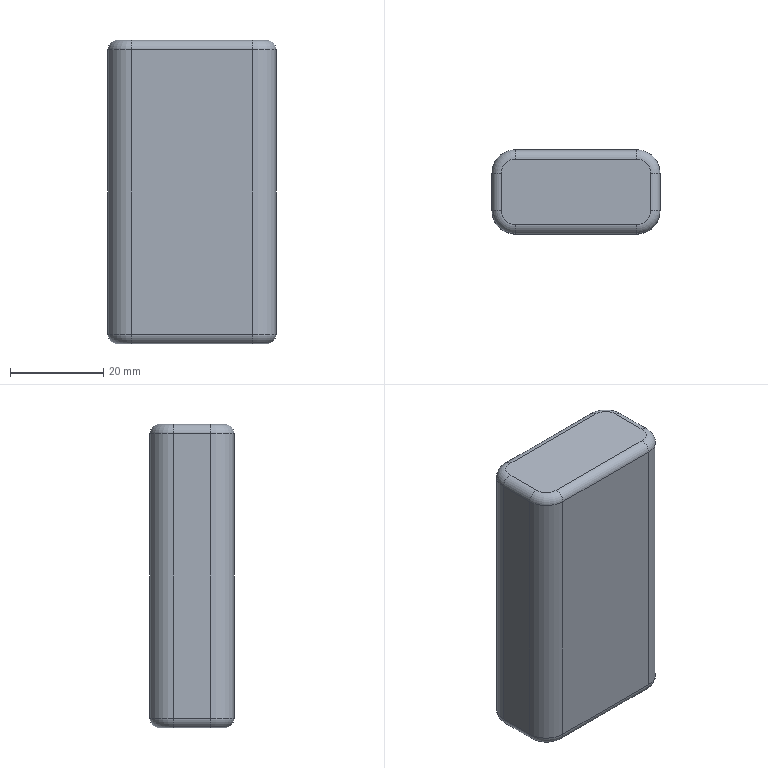Part | SolidWorks | features Fillet 2, Extrusion 1 | 1 solid | 26 faces | box 36 x 18 x 65 mm | volume 40559 mm3 | cylinder 12 | torus 8 | plane 6 | commonest cylinder face diameters 4 x8 10 x4
STEP:
#1=CARTESIAN_POINT('',(18.,-4.,63.));
#2=VERTEX_POINT('',#1);
#3=CARTESIAN_POINT('',(18.,-4.,2.));
#4=VERTEX_POINT('',#3);
#5=CARTESIAN_POINT('',(18.,-4.,65.));
#6=DIRECTION('',(0.,0.,-1.));
#7=VECTOR('',#6,1000.);
#8=LINE('',#5,#7);
#9=EDGE_CURVE('',#2,#4,#8,.T.);
#10=ORIENTED_EDGE('',*,*,#9,.T.);
#11=CARTESIAN_POINT('',(18.,4.,2.));
#12=VERTEX_POINT('',#11);
#13=CARTESIAN_POINT('',(18.,9.,2.));
#14=DIRECTION('',(0.,1.,0.));
#15=VECTOR('',#14,1000.);
#16=LINE('',#13,#15);
#17=EDGE_CURVE('',#4,#12,#16,.T.);
#18=ORIENTED_EDGE('',*,*,#17,.T.);
#19=CARTESIAN_POINT('',(18.,4.,63.));
#20=VERTEX_POINT('',#19);
#21=CARTESIAN_POINT('',(18.,4.,65.));
#22=DIRECTION('',(0.,0.,1.));
#23=VECTOR('',#22,1000.);
#24=LINE('',#21,#23);
#25=EDGE_CURVE('',#12,#20,#24,.T.);
#26=ORIENTED_EDGE('',*,*,#25,.T.);
#27=CARTESIAN_POINT('',(18.,-4.,63.));
#28=DIRECTION('',(0.,-1.,0.));
#29=VECTOR('',#28,1000.);
#30=LINE('',#27,#29);
#31=EDGE_CURVE('',#20,#2,#30,.T.);
#32=ORIENTED_EDGE('',*,*,#31,.T.);
#33=EDGE_LOOP('',(#10,#18,#26,#32));
#34=FACE_OUTER_BOUND('',#33,.T.);
#35=CARTESIAN_POINT('',(18.,9.,65.));
#36=DIRECTION('',(-1.,0.,0.));
#37=DIRECTION('',(0.,0.,1.));
#38=AXIS2_PLACEMENT_3D('',#35,#36,#37);
#39=PLANE('',#38);
#40=ADVANCED_FACE('',(#34),#39,.F.);
#41=CARTESIAN_POINT('',(13.,9.,63.));
#42=VERTEX_POINT('',#41);
#43=CARTESIAN_POINT('',(13.,9.,2.));
#44=VERTEX_POINT('',#43);
#45=CARTESIAN_POINT('',(13.,9.,65.));
#46=DIRECTION('',(0.,0.,-1.));
#47=VECTOR('',#46,1000.);
#48=LINE('',#45,#47);
#49=EDGE_CURVE('',#42,#44,#48,.T.);
#50=ORIENTED_EDGE('',*,*,#49,.T.);
#51=CARTESIAN_POINT('',(-13.,9.,2.));
#52=VERTEX_POINT('',#51);
#53=CARTESIAN_POINT('',(-18.,9.,2.));
#54=DIRECTION('',(-1.,0.,0.));
#55=VECTOR('',#54,1000.);
#56=LINE('',#53,#55);
#57=EDGE_CURVE('',#44,#52,#56,.T.);
#58=ORIENTED_EDGE('',*,*,#57,.T.);
#59=CARTESIAN_POINT('',(-13.,9.,63.));
#60=VERTEX_POINT('',#59);
#61=CARTESIAN_POINT('',(-13.,9.,65.));
#62=DIRECTION('',(0.,0.,1.));
#63=VECTOR('',#62,1000.);
#64=LINE('',#61,#63);
#65=EDGE_CURVE('',#52,#60,#64,.T.);
#66=ORIENTED_EDGE('',*,*,#65,.T.);
#67=CARTESIAN_POINT('',(13.,9.,63.));
#68=DIRECTION('',(1.,0.,0.));
#69=VECTOR('',#68,1000.);
#70=LINE('',#67,#69);
#71=EDGE_CURVE('',#60,#42,#70,.T.);
#72=ORIENTED_EDGE('',*,*,#71,.T.);
#73=EDGE_LOOP('',(#50,#58,#66,#72));
#74=FACE_OUTER_BOUND('',#73,.T.);
#75=CARTESIAN_POINT('',(-18.,9.,65.));
#76=DIRECTION('',(0.,-1.,0.));
#77=DIRECTION('',(0.,0.,-1.));
#78=AXIS2_PLACEMENT_3D('',#75,#76,#77);
#79=PLANE('',#78);
#80=ADVANCED_FACE('',(#74),#79,.F.);
#81=CARTESIAN_POINT('',(-18.,4.,63.));
#82=VERTEX_POINT('',#81);
#83=CARTESIAN_POINT('',(-18.,4.,2.));
#84=VERTEX_POINT('',#83);
#85=CARTESIAN_POINT('',(-18.,4.,65.));
#86=DIRECTION('',(0.,0.,-1.));
#87=VECTOR('',#86,1000.);
#88=LINE('',#85,#87);
#89=EDGE_CURVE('',#82,#84,#88,.T.);
#90=ORIENTED_EDGE('',*,*,#89,.T.);
#91=CARTESIAN_POINT('',(-18.,-4.,2.));
#92=VERTEX_POINT('',#91);
#93=CARTESIAN_POINT('',(-18.,9.,2.));
#94=DIRECTION('',(0.,-1.,0.));
#95=VECTOR('',#94,1000.);
#96=LINE('',#93,#95);
#97=EDGE_CURVE('',#84,#92,#96,.T.);
#98=ORIENTED_EDGE('',*,*,#97,.T.);
#99=CARTESIAN_POINT('',(-18.,-4.,63.));
#100=VERTEX_POINT('',#99);
#101=CARTESIAN_POINT('',(-18.,-4.,65.));
#102=DIRECTION('',(0.,0.,1.));
#103=VECTOR('',#102,1000.);
#104=LINE('',#101,#103);
#105=EDGE_CURVE('',#92,#100,#104,.T.);
#106=ORIENTED_EDGE('',*,*,#105,.T.);
#107=CARTESIAN_POINT('',(-18.,4.,63.));
#108=DIRECTION('',(0.,1.,0.));
#109=VECTOR('',#108,1000.);
#110=LINE('',#107,#109);
#111=EDGE_CURVE('',#100,#82,#110,.T.);
#112=ORIENTED_EDGE('',*,*,#111,.T.);
#113=EDGE_LOOP('',(#90,#98,#106,#112));
#114=FACE_OUTER_BOUND('',#113,.T.);
#115=CARTESIAN_POINT('',(-18.,9.,65.));
#116=DIRECTION('',(1.,0.,0.));
#117=DIRECTION('',(0.,0.,-1.));
#118=AXIS2_PLACEMENT_3D('',#115,#116,#117);
#119=PLANE('',#118);
#120=ADVANCED_FACE('',(#114),#119,.F.);
#121=CARTESIAN_POINT('',(-13.,-9.,63.));
#122=VERTEX_POINT('',#121);
#123=CARTESIAN_POINT('',(-13.,-9.,2.));
#124=VERTEX_POINT('',#123);
#125=CARTESIAN_POINT('',(-13.,-9.,65.));
#126=DIRECTION('',(0.,0.,-1.));
#127=VECTOR('',#126,1000.);
#128=LINE('',#125,#127);
#129=EDGE_CURVE('',#122,#124,#128,.T.);
#130=ORIENTED_EDGE('',*,*,#129,.T.);
#131=CARTESIAN_POINT('',(13.,-9.,2.));
#132=VERTEX_POINT('',#131);
#133=CARTESIAN_POINT('',(-18.,-9.,2.));
#134=DIRECTION('',(1.,0.,0.));
#135=VECTOR('',#134,1000.);
#136=LINE('',#133,#135);
#137=EDGE_CURVE('',#124,#132,#136,.T.);
#138=ORIENTED_EDGE('',*,*,#137,.T.);
#139=CARTESIAN_POINT('',(13.,-9.,63.));
#140=VERTEX_POINT('',#139);
#141=CARTESIAN_POINT('',(13.,-9.,65.));
#142=DIRECTION('',(0.,0.,1.));
#143=VECTOR('',#142,1000.);
#144=LINE('',#141,#143);
#145=EDGE_CURVE('',#132,#140,#144,.T.);
#146=ORIENTED_EDGE('',*,*,#145,.T.);
#147=CARTESIAN_POINT('',(-13.,-9.,63.));
#148=DIRECTION('',(-1.,0.,0.));
#149=VECTOR('',#148,1000.);
#150=LINE('',#147,#149);
#151=EDGE_CURVE('',#140,#122,#150,.T.);
#152=ORIENTED_EDGE('',*,*,#151,.T.);
#153=EDGE_LOOP('',(#130,#138,#146,#152));
#154=FACE_OUTER_BOUND('',#153,.T.);
#155=CARTESIAN_POINT('',(-18.,-9.,65.));
#156=DIRECTION('',(0.,1.,0.));
#157=DIRECTION('',(0.,0.,1.));
#158=AXIS2_PLACEMENT_3D('',#155,#156,#157);
#159=PLANE('',#158);
#160=ADVANCED_FACE('',(#154),#159,.F.);
#161=CARTESIAN_POINT('',(13.,7.,65.));
#162=VERTEX_POINT('',#161);
#163=CARTESIAN_POINT('',(-13.,7.,65.));
#164=VERTEX_POINT('',#163);
#165=CARTESIAN_POINT('',(-13.,7.,65.));
#166=DIRECTION('',(-1.,0.,0.));
#167=VECTOR('',#166,1000.);
#168=LINE('',#165,#167);
#169=EDGE_CURVE('',#162,#164,#168,.T.);
#170=ORIENTED_EDGE('',*,*,#169,.T.);
#171=CARTESIAN_POINT('',(-16.,4.,65.));
#172=VERTEX_POINT('',#171);
#173=CARTESIAN_POINT('',(-13.,4.,65.));
#174=DIRECTION('',(0.,0.,1.));
#175=DIRECTION('',(1.,0.,0.));
#176=AXIS2_PLACEMENT_3D('',#173,#174,#175);
#177=CIRCLE('',#176,3.);
#178=EDGE_CURVE('',#164,#172,#177,.T.);
#179=ORIENTED_EDGE('',*,*,#178,.T.);
#180=CARTESIAN_POINT('',(-16.,-4.,65.));
#181=VERTEX_POINT('',#180);
#182=CARTESIAN_POINT('',(-16.,-4.,65.));
#183=DIRECTION('',(0.,-1.,0.));
#184=VECTOR('',#183,1000.);
#185=LINE('',#182,#184);
#186=EDGE_CURVE('',#172,#181,#185,.T.);
#187=ORIENTED_EDGE('',*,*,#186,.T.);
#188=CARTESIAN_POINT('',(-13.,-7.,65.));
#189=VERTEX_POINT('',#188);
#190=CARTESIAN_POINT('',(-13.,-4.,65.));
#191=DIRECTION('',(0.,0.,1.));
#192=DIRECTION('',(1.,0.,0.));
#193=AXIS2_PLACEMENT_3D('',#190,#191,#192);
#194=CIRCLE('',#193,3.);
#195=EDGE_CURVE('',#181,#189,#194,.T.);
#196=ORIENTED_EDGE('',*,*,#195,.T.);
#197=CARTESIAN_POINT('',(13.,-7.,65.));
#198=VERTEX_POINT('',#197);
#199=CARTESIAN_POINT('',(13.,-7.,65.));
#200=DIRECTION('',(1.,0.,0.));
#201=VECTOR('',#200,1000.);
#202=LINE('',#199,#201);
#203=EDGE_CURVE('',#189,#198,#202,.T.);
#204=ORIENTED_EDGE('',*,*,#203,.T.);
#205=CARTESIAN_POINT('',(16.,-4.,65.));
#206=VERTEX_POINT('',#205);
#207=CARTESIAN_POINT('',(13.,-4.,65.));
#208=DIRECTION('',(0.,0.,1.));
#209=DIRECTION('',(1.,0.,0.));
#210=AXIS2_PLACEMENT_3D('',#207,#208,#209);
#211=CIRCLE('',#210,3.);
#212=EDGE_CURVE('',#198,#206,#211,.T.);
#213=ORIENTED_EDGE('',*,*,#212,.T.);
#214=CARTESIAN_POINT('',(16.,4.,65.));
#215=VERTEX_POINT('',#214);
#216=CARTESIAN_POINT('',(16.,4.,65.));
#217=DIRECTION('',(0.,1.,0.));
#218=VECTOR('',#217,1000.);
#219=LINE('',#216,#218);
#220=EDGE_CURVE('',#206,#215,#219,.T.);
#221=ORIENTED_EDGE('',*,*,#220,.T.);
#222=CARTESIAN_POINT('',(13.,4.,65.));
#223=DIRECTION('',(0.,0.,1.));
#224=DIRECTION('',(1.,0.,0.));
#225=AXIS2_PLACEMENT_3D('',#222,#223,#224);
#226=CIRCLE('',#225,3.);
#227=EDGE_CURVE('',#215,#162,#226,.T.);
#228=ORIENTED_EDGE('',*,*,#227,.T.);
#229=EDGE_LOOP('',(#170,#179,#187,#196,#204,#213,#221,#228));
#230=FACE_OUTER_BOUND('',#229,.T.);
#231=CARTESIAN_POINT('',(0.,0.,65.));
#232=DIRECTION('',(0.,0.,1.));
#233=DIRECTION('',(1.,0.,0.));
#234=AXIS2_PLACEMENT_3D('',#231,#232,#233);
#235=PLANE('',#234);
#236=ADVANCED_FACE('',(#230),#235,.T.);
#237=CARTESIAN_POINT('',(16.,4.,0.));
#238=VERTEX_POINT('',#237);
#239=CARTESIAN_POINT('',(16.,-4.,0.));
#240=VERTEX_POINT('',#239);
#241=CARTESIAN_POINT('',(16.,0.,0.));
#242=DIRECTION('',(0.,-1.,0.));
#243=VECTOR('',#242,1000.);
#244=LINE('',#241,#243);
#245=EDGE_CURVE('',#238,#240,#244,.T.);
#246=ORIENTED_EDGE('',*,*,#245,.T.);
#247=CARTESIAN_POINT('',(13.,-7.,0.));
#248=VERTEX_POINT('',#247);
#249=CARTESIAN_POINT('',(13.,-4.,0.));
#250=DIRECTION('',(0.,0.,-1.));
#251=DIRECTION('',(1.,0.,0.));
#252=AXIS2_PLACEMENT_3D('',#249,#250,#251);
#253=CIRCLE('',#252,3.);
#254=EDGE_CURVE('',#240,#248,#253,.T.);
#255=ORIENTED_EDGE('',*,*,#254,.T.);
#256=CARTESIAN_POINT('',(-13.,-7.,0.));
#257=VERTEX_POINT('',#256);
#258=CARTESIAN_POINT('',(0.,-7.,0.));
#259=DIRECTION('',(-1.,0.,0.));
#260=VECTOR('',#259,1000.);
#261=LINE('',#258,#260);
#262=EDGE_CURVE('',#248,#257,#261,.T.);
#263=ORIENTED_EDGE('',*,*,#262,.T.);
#264=CARTESIAN_POINT('',(-16.,-4.,0.));
#265=VERTEX_POINT('',#264);
#266=CARTESIAN_POINT('',(-13.,-4.,0.));
#267=DIRECTION('',(0.,0.,-1.));
#268=DIRECTION('',(1.,0.,0.));
#269=AXIS2_PLACEMENT_3D('',#266,#267,#268);
#270=CIRCLE('',#269,3.);
#271=EDGE_CURVE('',#257,#265,#270,.T.);
#272=ORIENTED_EDGE('',*,*,#271,.T.);
#273=CARTESIAN_POINT('',(-16.,4.,0.));
#274=VERTEX_POINT('',#273);
#275=CARTESIAN_POINT('',(-16.,0.,0.));
#276=DIRECTION('',(0.,1.,0.));
#277=VECTOR('',#276,1000.);
#278=LINE('',#275,#277);
#279=EDGE_CURVE('',#265,#274,#278,.T.);
#280=ORIENTED_EDGE('',*,*,#279,.T.);
#281=CARTESIAN_POINT('',(-13.,7.,0.));
#282=VERTEX_POINT('',#281);
#283=CARTESIAN_POINT('',(-13.,4.,0.));
#284=DIRECTION('',(0.,0.,-1.));
#285=DIRECTION('',(1.,0.,0.));
#286=AXIS2_PLACEMENT_3D('',#283,#284,#285);
#287=CIRCLE('',#286,3.);
#288=EDGE_CURVE('',#274,#282,#287,.T.);
#289=ORIENTED_EDGE('',*,*,#288,.T.);
#290=CARTESIAN_POINT('',(13.,7.,0.));
#291=VERTEX_POINT('',#290);
#292=CARTESIAN_POINT('',(0.,7.,0.));
#293=DIRECTION('',(1.,0.,0.));
#294=VECTOR('',#293,1000.);
#295=LINE('',#292,#294);
#296=EDGE_CURVE('',#282,#291,#295,.T.);
#297=ORIENTED_EDGE('',*,*,#296,.T.);
#298=CARTESIAN_POINT('',(13.,4.,0.));
#299=DIRECTION('',(0.,0.,-1.));
#300=DIRECTION('',(1.,0.,0.));
#301=AXIS2_PLACEMENT_3D('',#298,#299,#300);
#302=CIRCLE('',#301,3.);
#303=EDGE_CURVE('',#291,#238,#302,.T.);
#304=ORIENTED_EDGE('',*,*,#303,.T.);
#305=EDGE_LOOP('',(#246,#255,#263,#272,#280,#289,#297,#304));
#306=FACE_OUTER_BOUND('',#305,.T.);
#307=CARTESIAN_POINT('',(0.,0.,0.));
#308=DIRECTION('',(0.,0.,1.));
#309=DIRECTION('',(1.,0.,0.));
#310=AXIS2_PLACEMENT_3D('',#307,#308,#309);
#311=PLANE('',#310);
#312=ADVANCED_FACE('',(#306),#311,.F.);
#313=ORIENTED_EDGE('',*,*,#105,.F.);
#314=CARTESIAN_POINT('',(-13.,-4.,2.));
#315=DIRECTION('',(0.,0.,1.));
#316=DIRECTION('',(1.,0.,0.));
#317=AXIS2_PLACEMENT_3D('',#314,#315,#316);
#318=CIRCLE('',#317,5.);
#319=EDGE_CURVE('',#92,#124,#318,.T.);
#320=ORIENTED_EDGE('',*,*,#319,.T.);
#321=ORIENTED_EDGE('',*,*,#129,.F.);
#322=CARTESIAN_POINT('',(-13.,-4.,63.));
#323=DIRECTION('',(0.,0.,-1.));
#324=DIRECTION('',(1.,0.,0.));
#325=AXIS2_PLACEMENT_3D('',#322,#323,#324);
#326=CIRCLE('',#325,5.);
#327=EDGE_CURVE('',#122,#100,#326,.T.);
#328=ORIENTED_EDGE('',*,*,#327,.T.);
#329=EDGE_LOOP('',(#313,#320,#321,#328));
#330=FACE_OUTER_BOUND('',#329,.T.);
#331=CARTESIAN_POINT('',(-13.,-4.,65.));
#332=DIRECTION('',(0.,0.,-1.));
#333=DIRECTION('',(-1.,0.,0.));
#334=AXIS2_PLACEMENT_3D('',#331,#332,#333);
#335=CYLINDRICAL_SURFACE('',#334,5.);
#336=ADVANCED_FACE('',(#330),#335,.T.);
#337=ORIENTED_EDGE('',*,*,#65,.F.);
#338=CARTESIAN_POINT('',(-13.,4.,2.));
#339=DIRECTION('',(0.,0.,1.));
#340=DIRECTION('',(1.,0.,0.));
#341=AXIS2_PLACEMENT_3D('',#338,#339,#340);
#342=CIRCLE('',#341,5.);
#343=EDGE_CURVE('',#52,#84,#342,.T.);
#344=ORIENTED_EDGE('',*,*,#343,.T.);
#345=ORIENTED_EDGE('',*,*,#89,.F.);
#346=CARTESIAN_POINT('',(-13.,4.,63.));
#347=DIRECTION('',(0.,0.,-1.));
#348=DIRECTION('',(1.,0.,0.));
#349=AXIS2_PLACEMENT_3D('',#346,#347,#348);
#350=CIRCLE('',#349,5.);
#351=EDGE_CURVE('',#82,#60,#350,.T.);
#352=ORIENTED_EDGE('',*,*,#351,.T.);
#353=EDGE_LOOP('',(#337,#344,#345,#352));
#354=FACE_OUTER_BOUND('',#353,.T.);
#355=CARTESIAN_POINT('',(-13.,4.,65.));
#356=DIRECTION('',(0.,0.,-1.));
#357=DIRECTION('',(-1.,0.,0.));
#358=AXIS2_PLACEMENT_3D('',#355,#356,#357);
#359=CYLINDRICAL_SURFACE('',#358,5.);
#360=ADVANCED_FACE('',(#354),#359,.T.);
#361=ORIENTED_EDGE('',*,*,#145,.F.);
#362=CARTESIAN_POINT('',(13.,-4.,2.));
#363=DIRECTION('',(0.,0.,1.));
#364=DIRECTION('',(1.,0.,0.));
#365=AXIS2_PLACEMENT_3D('',#362,#363,#364);
#366=CIRCLE('',#365,5.);
#367=EDGE_CURVE('',#132,#4,#366,.T.);
#368=ORIENTED_EDGE('',*,*,#367,.T.);
#369=ORIENTED_EDGE('',*,*,#9,.F.);
#370=CARTESIAN_POINT('',(13.,-4.,63.));
#371=DIRECTION('',(0.,0.,-1.));
#372=DIRECTION('',(1.,0.,0.));
#373=AXIS2_PLACEMENT_3D('',#370,#371,#372);
#374=CIRCLE('',#373,5.);
#375=EDGE_CURVE('',#2,#140,#374,.T.);
#376=ORIENTED_EDGE('',*,*,#375,.T.);
#377=EDGE_LOOP('',(#361,#368,#369,#376));
#378=FACE_OUTER_BOUND('',#377,.T.);
#379=CARTESIAN_POINT('',(13.,-4.,65.));
#380=DIRECTION('',(0.,0.,-1.));
#381=DIRECTION('',(-1.,0.,0.));
#382=AXIS2_PLACEMENT_3D('',#379,#380,#381);
#383=CYLINDRICAL_SURFACE('',#382,5.);
#384=ADVANCED_FACE('',(#378),#383,.T.);
#385=ORIENTED_EDGE('',*,*,#25,.F.);
#386=CARTESIAN_POINT('',(13.,4.,2.));
#387=DIRECTION('',(0.,0.,1.));
#388=DIRECTION('',(1.,0.,0.));
#389=AXIS2_PLACEMENT_3D('',#386,#387,#388);
#390=CIRCLE('',#389,5.);
#391=EDGE_CURVE('',#12,#44,#390,.T.);
#392=ORIENTED_EDGE('',*,*,#391,.T.);
#393=ORIENTED_EDGE('',*,*,#49,.F.);
#394=CARTESIAN_POINT('',(13.,4.,63.));
#395=DIRECTION('',(0.,0.,-1.));
#396=DIRECTION('',(1.,0.,0.));
#397=AXIS2_PLACEMENT_3D('',#394,#395,#396);
#398=CIRCLE('',#397,5.);
#399=EDGE_CURVE('',#42,#20,#398,.T.);
#400=ORIENTED_EDGE('',*,*,#399,.T.);
#401=EDGE_LOOP('',(#385,#392,#393,#400));
#402=FACE_OUTER_BOUND('',#401,.T.);
#403=CARTESIAN_POINT('',(13.,4.,65.));
#404=DIRECTION('',(0.,0.,-1.));
#405=DIRECTION('',(-1.,0.,0.));
#406=AXIS2_PLACEMENT_3D('',#403,#404,#405);
#407=CYLINDRICAL_SURFACE('',#406,5.);
#408=ADVANCED_FACE('',(#402),#407,.T.);
#409=CARTESIAN_POINT('',(-16.,4.,2.));
#410=DIRECTION('',(0.,-1.,0.));
#411=DIRECTION('',(0.,0.,-1.));
#412=AXIS2_PLACEMENT_3D('',#409,#410,#411);
#413=CIRCLE('',#412,2.);
#414=EDGE_CURVE('',#84,#274,#413,.T.);
#415=ORIENTED_EDGE('',*,*,#414,.F.);
#416=ORIENTED_EDGE('',*,*,#343,.F.);
#417=CARTESIAN_POINT('',(-13.,7.,2.));
#418=DIRECTION('',(1.,0.,0.));
#419=DIRECTION('',(0.,0.,-1.));
#420=AXIS2_PLACEMENT_3D('',#417,#418,#419);
#421=CIRCLE('',#420,2.);
#422=EDGE_CURVE('',#282,#52,#421,.T.);
#423=ORIENTED_EDGE('',*,*,#422,.F.);
#424=ORIENTED_EDGE('',*,*,#288,.F.);
#425=EDGE_LOOP('',(#415,#416,#423,#424));
#426=FACE_OUTER_BOUND('',#425,.T.);
#427=CARTESIAN_POINT('',(-13.,4.,2.));
#428=DIRECTION('',(0.,0.,1.));
#429=DIRECTION('',(1.,0.,0.));
#430=AXIS2_PLACEMENT_3D('',#427,#428,#429);
#431=TOROIDAL_SURFACE('',#430,3.,2.);
#432=ADVANCED_FACE('',(#426),#431,.T.);
#433=ORIENTED_EDGE('',*,*,#422,.T.);
#434=ORIENTED_EDGE('',*,*,#57,.F.);
#435=CARTESIAN_POINT('',(13.,7.,2.));
#436=DIRECTION('',(1.,0.,0.));
#437=DIRECTION('',(0.,0.,-1.));
#438=AXIS2_PLACEMENT_3D('',#435,#436,#437);
#439=CIRCLE('',#438,2.);
#440=EDGE_CURVE('',#291,#44,#439,.T.);
#441=ORIENTED_EDGE('',*,*,#440,.F.);
#442=ORIENTED_EDGE('',*,*,#296,.F.);
#443=EDGE_LOOP('',(#433,#434,#441,#442));
#444=FACE_OUTER_BOUND('',#443,.T.);
#445=CARTESIAN_POINT('',(-18.,7.,2.));
#446=DIRECTION('',(-1.,0.,0.));
#447=DIRECTION('',(0.,0.,1.));
#448=AXIS2_PLACEMENT_3D('',#445,#446,#447);
#449=CYLINDRICAL_SURFACE('',#448,2.);
#450=ADVANCED_FACE('',(#444),#449,.T.);
#451=ORIENTED_EDGE('',*,*,#414,.T.);
#452=ORIENTED_EDGE('',*,*,#279,.F.);
#453=CARTESIAN_POINT('',(-16.,-4.,2.));
#454=DIRECTION('',(0.,-1.,0.));
#455=DIRECTION('',(0.,0.,-1.));
#456=AXIS2_PLACEMENT_3D('',#453,#454,#455);
#457=CIRCLE('',#456,2.);
#458=EDGE_CURVE('',#92,#265,#457,.T.);
#459=ORIENTED_EDGE('',*,*,#458,.F.);
#460=ORIENTED_EDGE('',*,*,#97,.F.);
#461=EDGE_LOOP('',(#451,#452,#459,#460));
#462=FACE_OUTER_BOUND('',#461,.T.);
#463=CARTESIAN_POINT('',(-16.,9.,2.));
#464=DIRECTION('',(0.,-1.,0.));
#465=DIRECTION('',(0.,0.,-1.));
#466=AXIS2_PLACEMENT_3D('',#463,#464,#465);
#467=CYLINDRICAL_SURFACE('',#466,2.);
#468=ADVANCED_FACE('',(#462),#467,.T.);
#469=ORIENTED_EDGE('',*,*,#440,.T.);
#470=ORIENTED_EDGE('',*,*,#391,.F.);
#471=CARTESIAN_POINT('',(16.,4.,2.));
#472=DIRECTION('',(0.,-1.,0.));
#473=DIRECTION('',(0.,0.,-1.));
#474=AXIS2_PLACEMENT_3D('',#471,#472,#473);
#475=CIRCLE('',#474,2.);
#476=EDGE_CURVE('',#238,#12,#475,.T.);
#477=ORIENTED_EDGE('',*,*,#476,.F.);
#478=ORIENTED_EDGE('',*,*,#303,.F.);
#479=EDGE_LOOP('',(#469,#470,#477,#478));
#480=FACE_OUTER_BOUND('',#479,.T.);
#481=CARTESIAN_POINT('',(13.,4.,2.));
#482=DIRECTION('',(0.,0.,1.));
#483=DIRECTION('',(1.,0.,0.));
#484=AXIS2_PLACEMENT_3D('',#481,#482,#483);
#485=TOROIDAL_SURFACE('',#484,3.,2.);
#486=ADVANCED_FACE('',(#480),#485,.T.);
#487=ORIENTED_EDGE('',*,*,#458,.T.);
#488=ORIENTED_EDGE('',*,*,#271,.F.);
#489=CARTESIAN_POINT('',(-13.,-7.,2.));
#490=DIRECTION('',(1.,0.,0.));
#491=DIRECTION('',(0.,0.,-1.));
#492=AXIS2_PLACEMENT_3D('',#489,#490,#491);
#493=CIRCLE('',#492,2.);
#494=EDGE_CURVE('',#124,#257,#493,.T.);
#495=ORIENTED_EDGE('',*,*,#494,.F.);
#496=ORIENTED_EDGE('',*,*,#319,.F.);
#497=EDGE_LOOP('',(#487,#488,#495,#496));
#498=FACE_OUTER_BOUND('',#497,.T.);
#499=CARTESIAN_POINT('',(-13.,-4.,2.));
#500=DIRECTION('',(0.,0.,1.));
#501=DIRECTION('',(1.,0.,0.));
#502=AXIS2_PLACEMENT_3D('',#499,#500,#501);
#503=TOROIDAL_SURFACE('',#502,3.,2.);
#504=ADVANCED_FACE('',(#498),#503,.T.);
#505=ORIENTED_EDGE('',*,*,#476,.T.);
#506=ORIENTED_EDGE('',*,*,#17,.F.);
#507=CARTESIAN_POINT('',(16.,-4.,2.));
#508=DIRECTION('',(0.,-1.,0.));
#509=DIRECTION('',(0.,0.,-1.));
#510=AXIS2_PLACEMENT_3D('',#507,#508,#509);
#511=CIRCLE('',#510,2.);
#512=EDGE_CURVE('',#240,#4,#511,.T.);
#513=ORIENTED_EDGE('',*,*,#512,.F.);
#514=ORIENTED_EDGE('',*,*,#245,.F.);
#515=EDGE_LOOP('',(#505,#506,#513,#514));
#516=FACE_OUTER_BOUND('',#515,.T.);
#517=CARTESIAN_POINT('',(16.,9.,2.));
#518=DIRECTION('',(0.,1.,0.));
#519=DIRECTION('',(0.,0.,1.));
#520=AXIS2_PLACEMENT_3D('',#517,#518,#519);
#521=CYLINDRICAL_SURFACE('',#520,2.);
#522=ADVANCED_FACE('',(#516),#521,.T.);
#523=ORIENTED_EDGE('',*,*,#494,.T.);
#524=ORIENTED_EDGE('',*,*,#262,.F.);
#525=CARTESIAN_POINT('',(13.,-7.,2.));
#526=DIRECTION('',(1.,0.,0.));
#527=DIRECTION('',(0.,0.,-1.));
#528=AXIS2_PLACEMENT_3D('',#525,#526,#527);
#529=CIRCLE('',#528,2.);
#530=EDGE_CURVE('',#132,#248,#529,.T.);
#531=ORIENTED_EDGE('',*,*,#530,.F.);
#532=ORIENTED_EDGE('',*,*,#137,.F.);
#533=EDGE_LOOP('',(#523,#524,#531,#532));
#534=FACE_OUTER_BOUND('',#533,.T.);
#535=CARTESIAN_POINT('',(-18.,-7.,2.));
#536=DIRECTION('',(1.,0.,0.));
#537=DIRECTION('',(0.,0.,-1.));
#538=AXIS2_PLACEMENT_3D('',#535,#536,#537);
#539=CYLINDRICAL_SURFACE('',#538,2.);
#540=ADVANCED_FACE('',(#534),#539,.T.);
#541=ORIENTED_EDGE('',*,*,#512,.T.);
#542=ORIENTED_EDGE('',*,*,#367,.F.);
#543=ORIENTED_EDGE('',*,*,#530,.T.);
#544=ORIENTED_EDGE('',*,*,#254,.F.);
#545=EDGE_LOOP('',(#541,#542,#543,#544));
#546=FACE_OUTER_BOUND('',#545,.T.);
#547=CARTESIAN_POINT('',(13.,-4.,2.));
#548=DIRECTION('',(0.,0.,1.));
#549=DIRECTION('',(1.,0.,0.));
#550=AXIS2_PLACEMENT_3D('',#547,#548,#549);
#551=TOROIDAL_SURFACE('',#550,3.,2.);
#552=ADVANCED_FACE('',(#546),#551,.T.);
#553=CARTESIAN_POINT('',(13.,-7.,63.));
#554=DIRECTION('',(-1.,0.,0.));
#555=DIRECTION('',(0.,0.,1.));
#556=AXIS2_PLACEMENT_3D('',#553,#554,#555);
#557=CIRCLE('',#556,2.);
#558=EDGE_CURVE('',#140,#198,#557,.T.);
#559=ORIENTED_EDGE('',*,*,#558,.F.);
#560=ORIENTED_EDGE('',*,*,#375,.F.);
#561=CARTESIAN_POINT('',(16.,-4.,63.));
#562=DIRECTION('',(0.,1.,0.));
#563=DIRECTION('',(0.,0.,1.));
#564=AXIS2_PLACEMENT_3D('',#561,#562,#563);
#565=CIRCLE('',#564,2.);
#566=EDGE_CURVE('',#206,#2,#565,.T.);
#567=ORIENTED_EDGE('',*,*,#566,.F.);
#568=ORIENTED_EDGE('',*,*,#212,.F.);
#569=EDGE_LOOP('',(#559,#560,#567,#568));
#570=FACE_OUTER_BOUND('',#569,.T.);
#571=CARTESIAN_POINT('',(13.,-4.,63.));
#572=DIRECTION('',(0.,0.,1.));
#573=DIRECTION('',(1.,0.,0.));
#574=AXIS2_PLACEMENT_3D('',#571,#572,#573);
#575=TOROIDAL_SURFACE('',#574,3.,2.);
#576=ADVANCED_FACE('',(#570),#575,.T.);
#577=ORIENTED_EDGE('',*,*,#566,.T.);
#578=ORIENTED_EDGE('',*,*,#31,.F.);
#579=CARTESIAN_POINT('',(16.,4.,63.));
#580=DIRECTION('',(0.,1.,0.));
#581=DIRECTION('',(0.,0.,1.));
#582=AXIS2_PLACEMENT_3D('',#579,#580,#581);
#583=CIRCLE('',#582,2.);
#584=EDGE_CURVE('',#215,#20,#583,.T.);
#585=ORIENTED_EDGE('',*,*,#584,.F.);
#586=ORIENTED_EDGE('',*,*,#220,.F.);
#587=EDGE_LOOP('',(#577,#578,#585,#586));
#588=FACE_OUTER_BOUND('',#587,.T.);
#589=CARTESIAN_POINT('',(16.,0.,63.));
#590=DIRECTION('',(0.,-1.,0.));
#591=DIRECTION('',(0.,0.,-1.));
#592=AXIS2_PLACEMENT_3D('',#589,#590,#591);
#593=CYLINDRICAL_SURFACE('',#592,2.);
#594=ADVANCED_FACE('',(#588),#593,.T.);
#595=ORIENTED_EDGE('',*,*,#558,.T.);
#596=ORIENTED_EDGE('',*,*,#203,.F.);
#597=CARTESIAN_POINT('',(-13.,-7.,63.));
#598=DIRECTION('',(-1.,0.,0.));
#599=DIRECTION('',(0.,0.,1.));
#600=AXIS2_PLACEMENT_3D('',#597,#598,#599);
#601=CIRCLE('',#600,2.);
#602=EDGE_CURVE('',#122,#189,#601,.T.);
#603=ORIENTED_EDGE('',*,*,#602,.F.);
#604=ORIENTED_EDGE('',*,*,#151,.F.);
#605=EDGE_LOOP('',(#595,#596,#603,#604));
#606=FACE_OUTER_BOUND('',#605,.T.);
#607=CARTESIAN_POINT('',(0.,-7.,63.));
#608=DIRECTION('',(-1.,0.,0.));
#609=DIRECTION('',(0.,0.,1.));
#610=AXIS2_PLACEMENT_3D('',#607,#608,#609);
#611=CYLINDRICAL_SURFACE('',#610,2.);
#612=ADVANCED_FACE('',(#606),#611,.T.);
#613=ORIENTED_EDGE('',*,*,#584,.T.);
#614=ORIENTED_EDGE('',*,*,#399,.F.);
#615=CARTESIAN_POINT('',(13.,7.,63.));
#616=DIRECTION('',(-1.,0.,0.));
#617=DIRECTION('',(0.,0.,1.));
#618=AXIS2_PLACEMENT_3D('',#615,#616,#617);
#619=CIRCLE('',#618,2.);
#620=EDGE_CURVE('',#162,#42,#619,.T.);
#621=ORIENTED_EDGE('',*,*,#620,.F.);
#622=ORIENTED_EDGE('',*,*,#227,.F.);
#623=EDGE_LOOP('',(#613,#614,#621,#622));
#624=FACE_OUTER_BOUND('',#623,.T.);
#625=CARTESIAN_POINT('',(13.,4.,63.));
#626=DIRECTION('',(0.,0.,1.));
#627=DIRECTION('',(1.,0.,0.));
#628=AXIS2_PLACEMENT_3D('',#625,#626,#627);
#629=TOROIDAL_SURFACE('',#628,3.,2.);
#630=ADVANCED_FACE('',(#624),#629,.T.);
#631=ORIENTED_EDGE('',*,*,#602,.T.);
#632=ORIENTED_EDGE('',*,*,#195,.F.);
#633=CARTESIAN_POINT('',(-16.,-4.,63.));
#634=DIRECTION('',(0.,1.,0.));
#635=DIRECTION('',(0.,0.,1.));
#636=AXIS2_PLACEMENT_3D('',#633,#634,#635);
#637=CIRCLE('',#636,2.);
#638=EDGE_CURVE('',#100,#181,#637,.T.);
#639=ORIENTED_EDGE('',*,*,#638,.F.);
#640=ORIENTED_EDGE('',*,*,#327,.F.);
#641=EDGE_LOOP('',(#631,#632,#639,#640));
#642=FACE_OUTER_BOUND('',#641,.T.);
#643=CARTESIAN_POINT('',(-13.,-4.,63.));
#644=DIRECTION('',(0.,0.,1.));
#645=DIRECTION('',(1.,0.,0.));
#646=AXIS2_PLACEMENT_3D('',#643,#644,#645);
#647=TOROIDAL_SURFACE('',#646,3.,2.);
#648=ADVANCED_FACE('',(#642),#647,.T.);
#649=ORIENTED_EDGE('',*,*,#620,.T.);
#650=ORIENTED_EDGE('',*,*,#71,.F.);
#651=CARTESIAN_POINT('',(-13.,7.,63.));
#652=DIRECTION('',(-1.,0.,0.));
#653=DIRECTION('',(0.,0.,1.));
#654=AXIS2_PLACEMENT_3D('',#651,#652,#653);
#655=CIRCLE('',#654,2.);
#656=EDGE_CURVE('',#164,#60,#655,.T.);
#657=ORIENTED_EDGE('',*,*,#656,.F.);
#658=ORIENTED_EDGE('',*,*,#169,.F.);
#659=EDGE_LOOP('',(#649,#650,#657,#658));
#660=FACE_OUTER_BOUND('',#659,.T.);
#661=CARTESIAN_POINT('',(0.,7.,63.));
#662=DIRECTION('',(1.,0.,0.));
#663=DIRECTION('',(0.,0.,-1.));
#664=AXIS2_PLACEMENT_3D('',#661,#662,#663);
#665=CYLINDRICAL_SURFACE('',#664,2.);
#666=ADVANCED_FACE('',(#660),#665,.T.);
#667=ORIENTED_EDGE('',*,*,#638,.T.);
#668=ORIENTED_EDGE('',*,*,#186,.F.);
#669=CARTESIAN_POINT('',(-16.,4.,63.));
#670=DIRECTION('',(0.,1.,0.));
#671=DIRECTION('',(0.,0.,1.));
#672=AXIS2_PLACEMENT_3D('',#669,#670,#671);
#673=CIRCLE('',#672,2.);
#674=EDGE_CURVE('',#82,#172,#673,.T.);
#675=ORIENTED_EDGE('',*,*,#674,.F.);
#676=ORIENTED_EDGE('',*,*,#111,.F.);
#677=EDGE_LOOP('',(#667,#668,#675,#676));
#678=FACE_OUTER_BOUND('',#677,.T.);
#679=CARTESIAN_POINT('',(-16.,0.,63.));
#680=DIRECTION('',(0.,1.,0.));
#681=DIRECTION('',(0.,0.,1.));
#682=AXIS2_PLACEMENT_3D('',#679,#680,#681);
#683=CYLINDRICAL_SURFACE('',#682,2.);
#684=ADVANCED_FACE('',(#678),#683,.T.);
#685=ORIENTED_EDGE('',*,*,#656,.T.);
#686=ORIENTED_EDGE('',*,*,#351,.F.);
#687=ORIENTED_EDGE('',*,*,#674,.T.);
#688=ORIENTED_EDGE('',*,*,#178,.F.);
#689=EDGE_LOOP('',(#685,#686,#687,#688));
#690=FACE_OUTER_BOUND('',#689,.T.);
#691=CARTESIAN_POINT('',(-13.,4.,63.));
#692=DIRECTION('',(0.,0.,1.));
#693=DIRECTION('',(1.,0.,0.));
#694=AXIS2_PLACEMENT_3D('',#691,#692,#693);
#695=TOROIDAL_SURFACE('',#694,3.,2.);
#696=ADVANCED_FACE('',(#690),#695,.T.);
#697=CLOSED_SHELL('',(#40,#80,#120,#160,#236,#312,#336,#360,#384,#408,#432,#450,#468,#486,#504,#522,#540,#552,#576,#594,#612,#630,#648,#666,#684,#696));
#698=MANIFOLD_SOLID_BREP('',#697);
#699=CARTESIAN_POINT('',(0.,0.,0.));
#700=DIRECTION('',(0.,0.,1.));
#701=DIRECTION('',(1.,0.,0.));
#702=AXIS2_PLACEMENT_3D('',#699,#700,#701);
#703=(LENGTH_UNIT()NAMED_UNIT(*)SI_UNIT(.MILLI.,.METRE.));
#704=UNCERTAINTY_MEASURE_WITH_UNIT(LENGTH_MEASURE(0.00001),#703,'','');
#705=(NAMED_UNIT(*)PLANE_ANGLE_UNIT()SI_UNIT($,.RADIAN.));
#706=(NAMED_UNIT(*)SI_UNIT($,.STERADIAN.)SOLID_ANGLE_UNIT());
#707=(GEOMETRIC_REPRESENTATION_CONTEXT(3)GLOBAL_UNCERTAINTY_ASSIGNED_CONTEXT((#704))GLOBAL_UNIT_ASSIGNED_CONTEXT((#703,#705,#706))REPRESENTATION_CONTEXT('',''));
#708=ADVANCED_BREP_SHAPE_REPRESENTATION('',(#698,#702),#707);